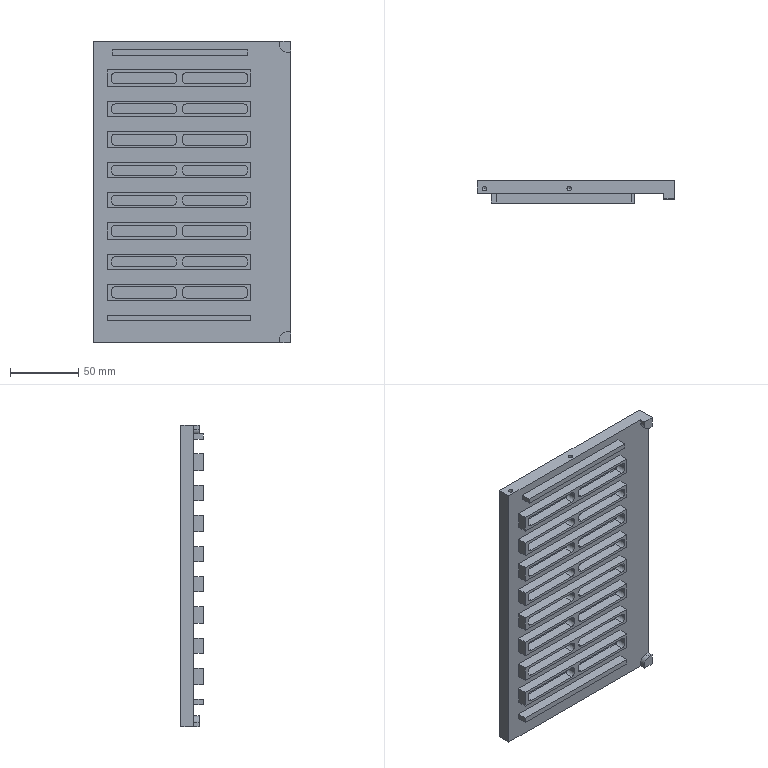NC program | NX | posted with a generic post | part box 144.5 x 16.5 x 221 mm
Lines 1 to 27 of 2050:
N10 G17 G21 G94 G90
(DRILLING_COPY_1 , TOOL : 倒角D6-90度)
N12 T11 M6
N14 G54
N16 G17 G0 G90 X4.95 Y-6. S2000 M3
N18 G43 Z20. H11
N20 G94 G81 G99 Z-0.9 F150. R3.
N22 X66.95
N24 G80
N26 G0 X66.95 Y-6. Z20.
N28 M5
(DRILLING_COPY_COPY_1 , TOOL : 钻头D3.3-45-73)
N30 T12 M6
N32 G54
N34 G17 G0 G90 X4.95 Y-6. S2000 M3
N36 G43 Z20. H12
N38 G94 G81 G99 Z-9.9 F200. R3.
N40 X66.95
N42 G80
N44 G0 X66.95 Y-6. Z20.
N46 M5